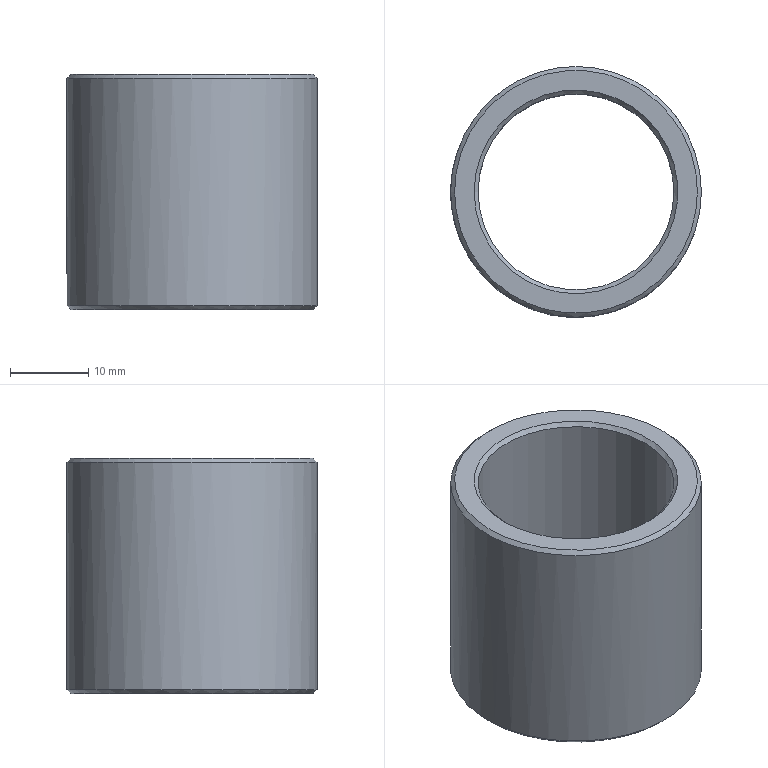Part | STEP file | solid 47 | 1 solid | 8 faces | box 32 x 32 x 30 mm | volume 9356 mm3 | cone 4 | plane 2 | cylinder 2 | commonest cylinder face diameters 25 x1 32 x1